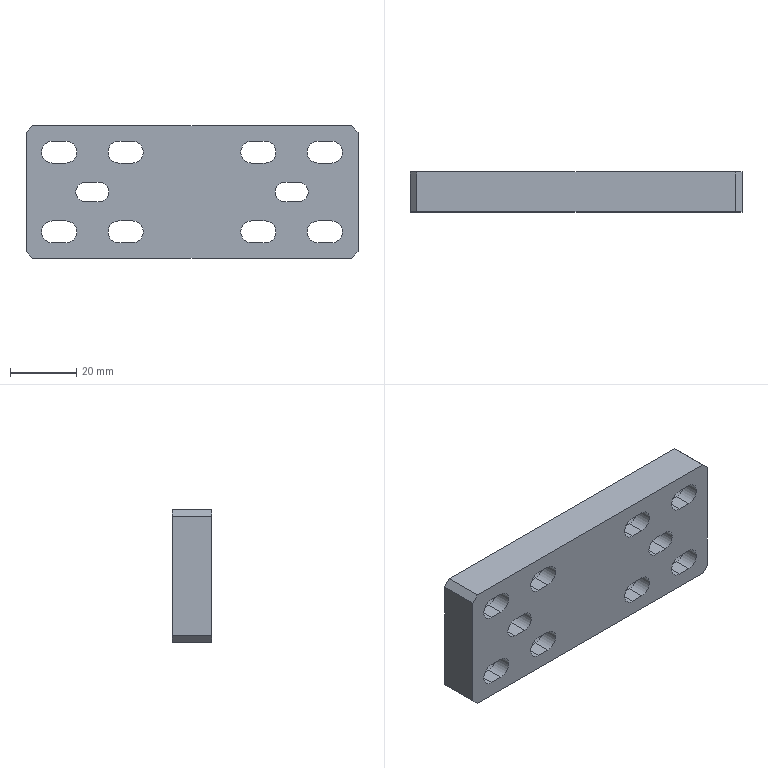Part | NX | features BREP 1 | 1 solid | 90 faces | box 100 x 12 x 40 mm | volume 36565 mm3 | plane 54 | cylinder 36 | commonest cylinder face diameters 6.6 x16 11 x16 6 x4